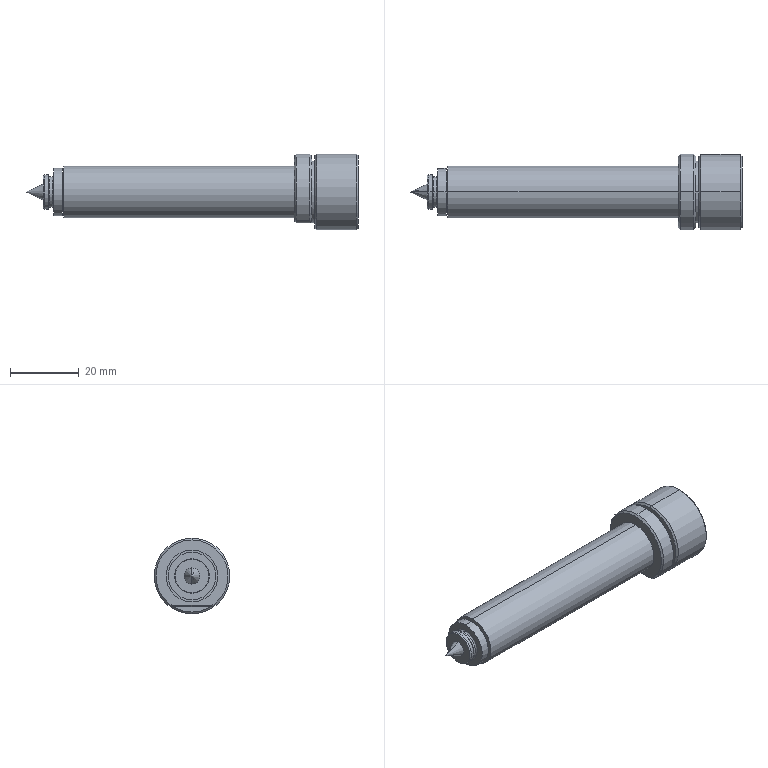Part | STEP file | BQM F BLOCO VMSMA C1=60mm GATE=1.25mm - TORRE | 1 solid | 57 faces | box 96.5 x 22 x 22 mm | volume 16557 mm3 | cylinder 20 | cone 17 | plane 14 | torus 6 | commonest cylinder face diameters 6 x4 10 x4 22 x4 9 x2 13.8 x2 15 x2